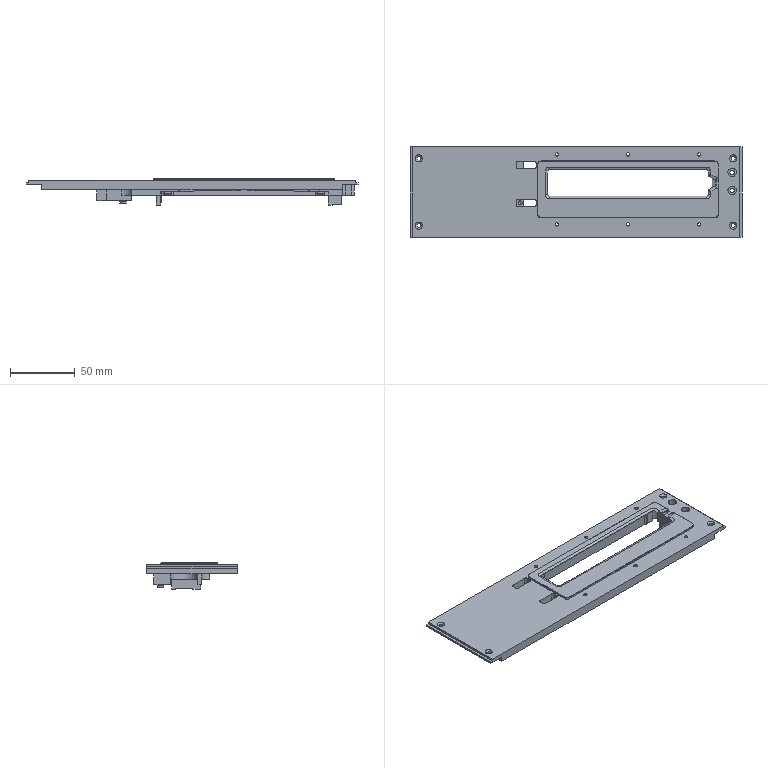NC program | NX | posted with a generic post | part box 256.6 x 70.3 x 20.422 mm
Lines 1 to 22 of 15201:
N10 G17 G21 G94 G90
(FLOOR_WALL , TOOL : D63)
N12 T01 M6
N14 G54
N16 G17 G0 G90 X-166.8 Y39.147 S6500 M3
N18 G43 Z30. H1
N20 Z3.
N22 G94 G1 Z0. F1250.
N24 X-163.8
N26 X163.8
N28 Y12.599
N30 X-163.8
N32 Y-13.95
N34 X163.8
N36 X166.8
N38 Z3.
N40 G0 Z30.
N42 M5